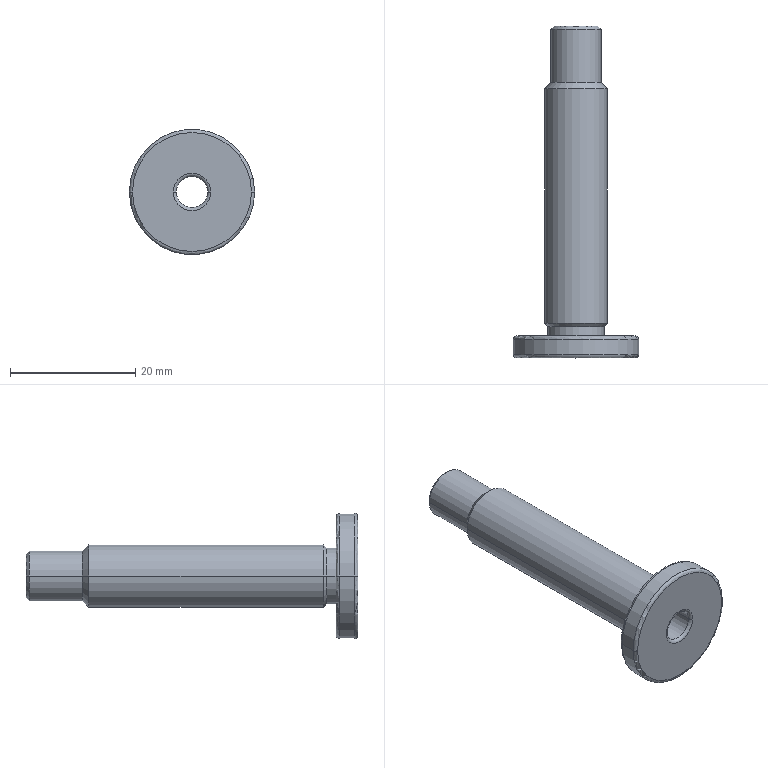Part | STEP file | VALVE_1PARTV11 | 1 solid | 30 faces | box 20 x 53 x 20 mm | volume 3450 mm3 | cone 10 | cylinder 10 | torus 6 | plane 4 | commonest cylinder face diameters 5 x2 8 x2 9 x2 10 x2 20 x2